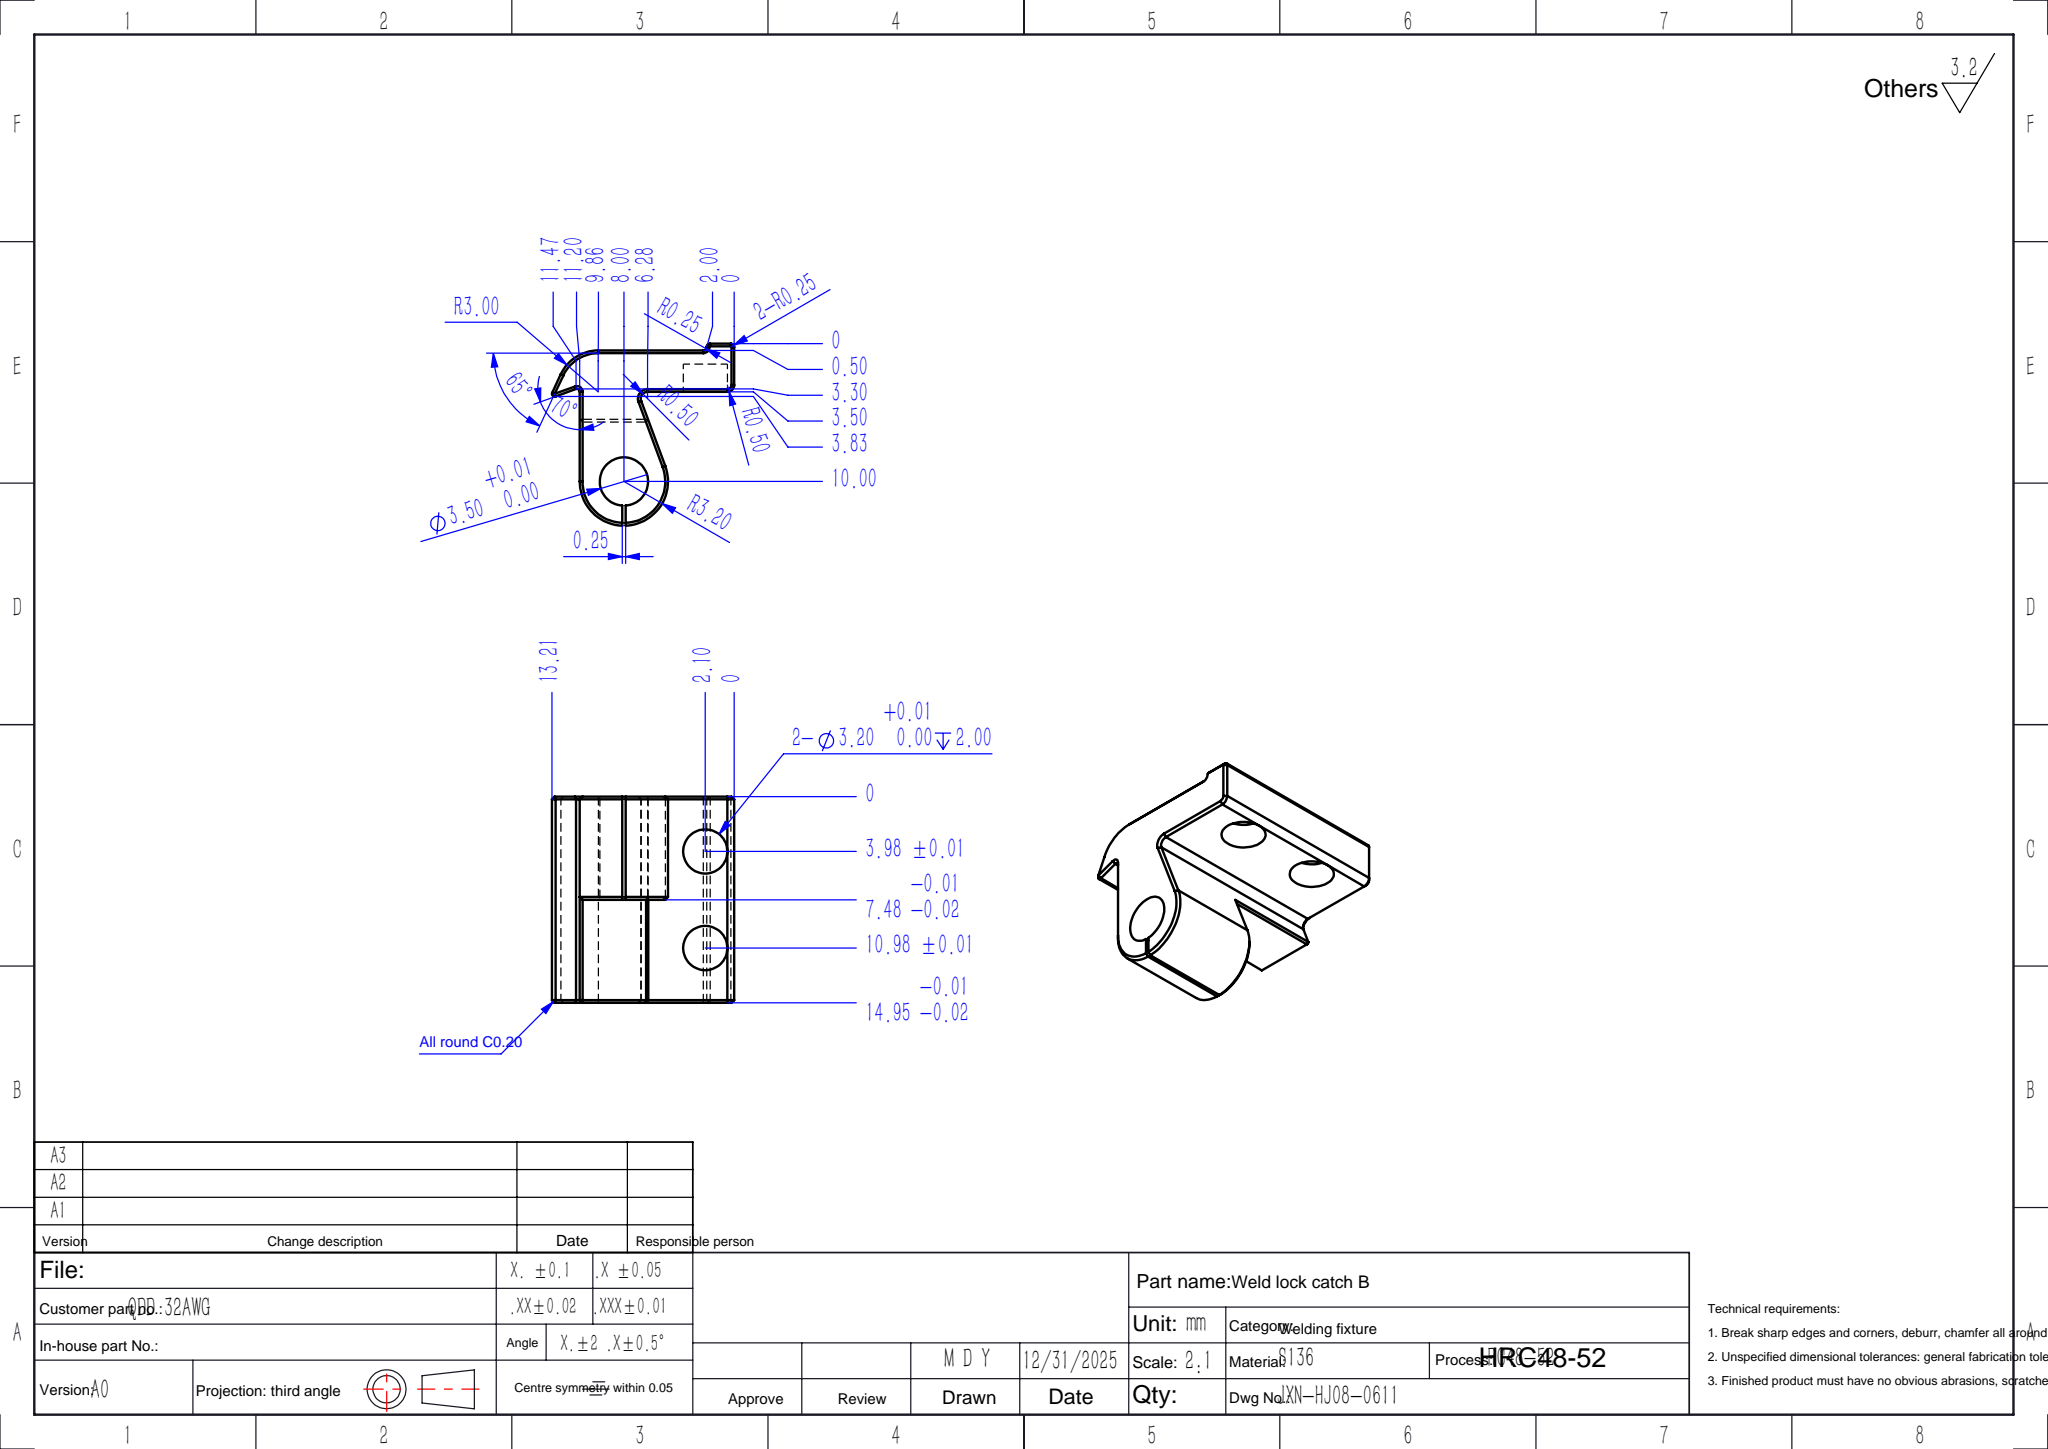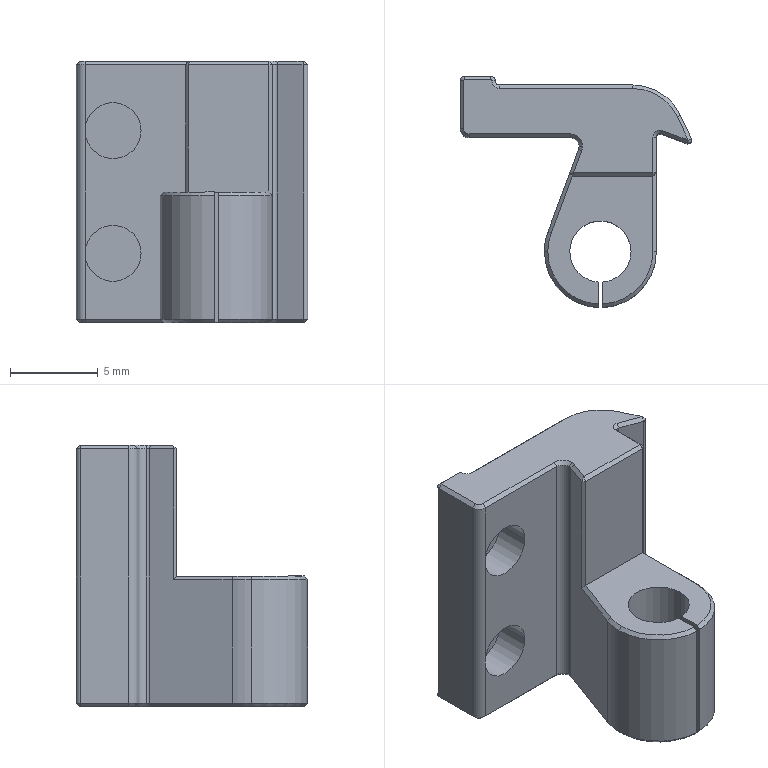Part | SolidWorks | features Fillet 6, ICE 5, Chamfer 1, Extrusion 1 | 1 solid | 81 faces | box 13.215 x 13.198 x 14.95 mm | volume 916.402 mm3 | plane 39 | cone 23 | cylinder 19 | commonest cylinder face diameters 3.2 x4 0.5 x3 1 x3 3.5 x3 6.4 x3 0.4 x2